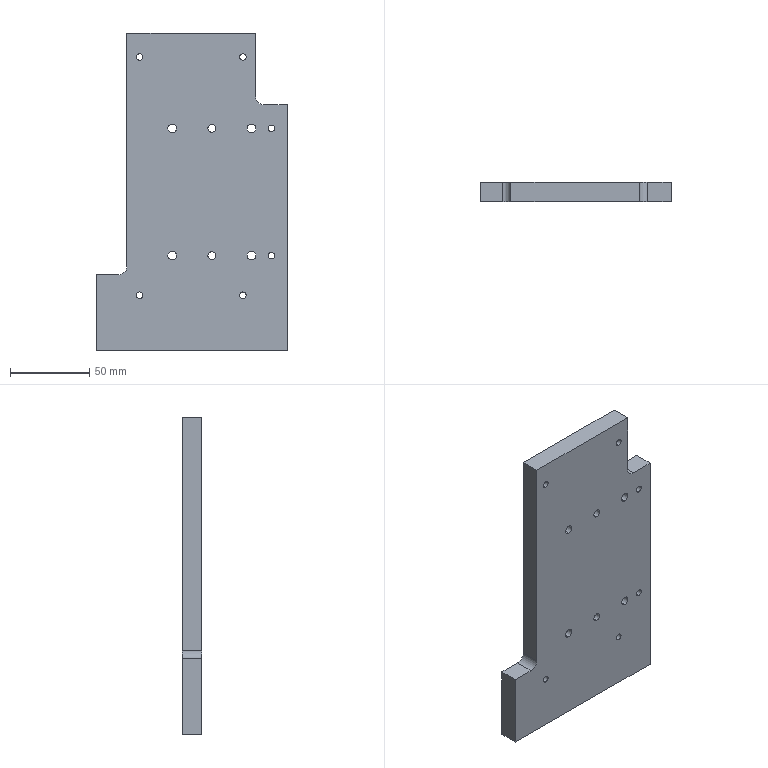Part | SolidWorks | features 3DProfileFeature 4, HoleWzd 4, Cut 3, Fillet 2, Boss 1, Extrusion 1 | 1 solid | 56 faces | box 120 x 12 x 200 mm | volume 238394 mm3 | cylinder 38 | plane 14 | cone 4 | commonest cylinder face diameters 4.2 x16 10 x10 5.5 x8 5 x4